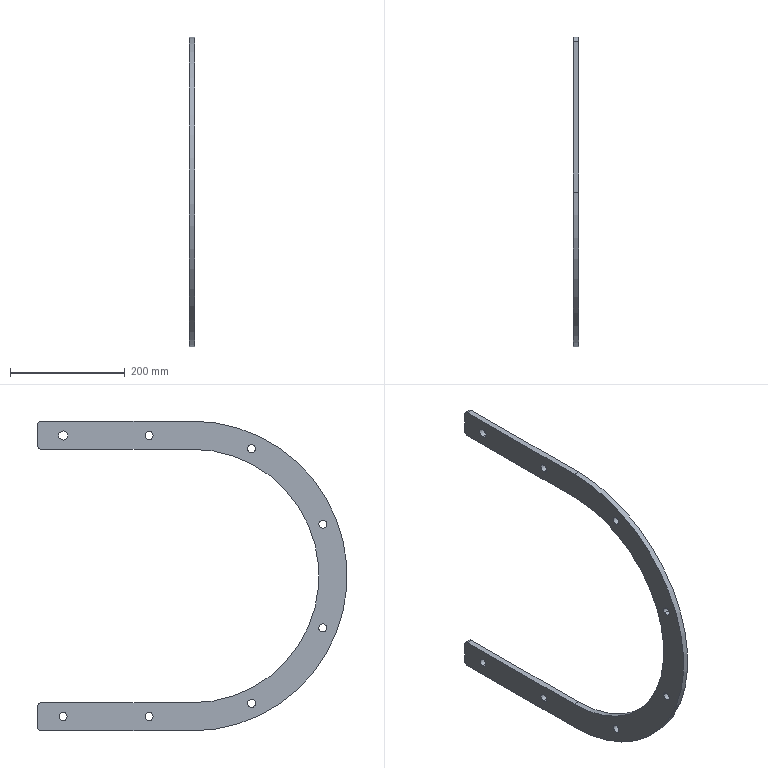Part | STEP file | Input 3 | 1 solid | 30 faces | box 10 x 540 x 540 mm | volume 629249 mm3 | cylinder 22 | plane 8 | commonest cylinder face diameters 14 x14 15 x4 16 x2 442 x1 540 x1